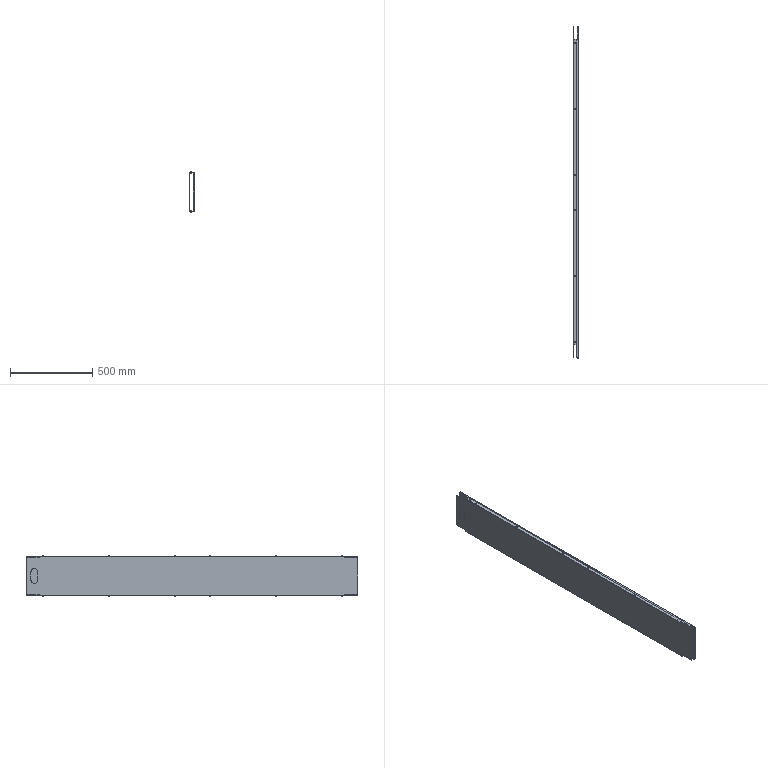Part | 16 solids | 303 faces | box 36 x 2016 x 253 mm | volume 1589479 mm3 | plane 164 | cylinder 139 | commonest cylinder face diameters 6 x32 6.2 x24 8 x24 8.2 x24 12 x24 0.4 x4